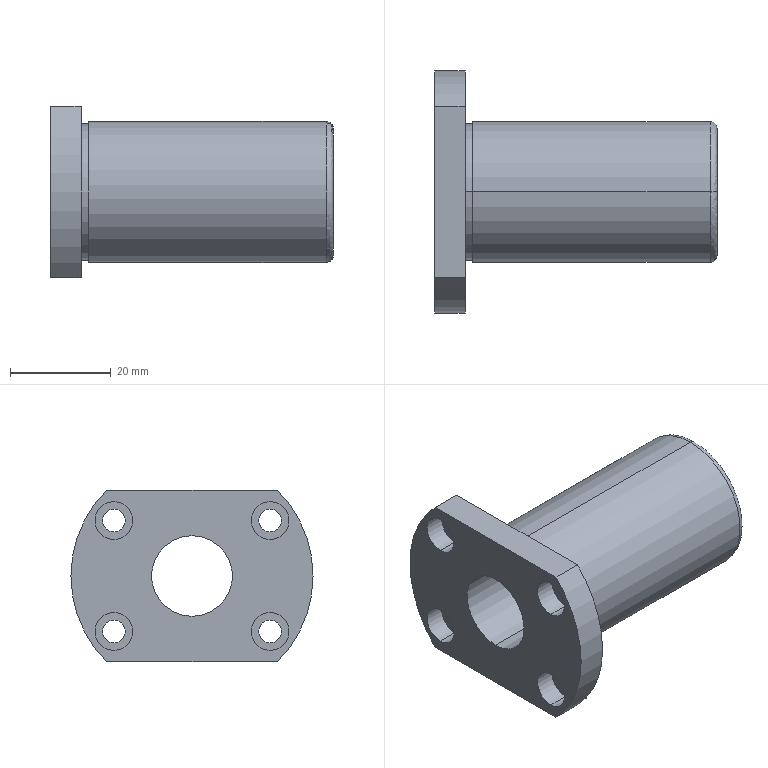Part | STEP file | LHFCD16 flanged linear bearing_LHFCD16 | 1 solid | 36 faces | box 56 x 48 x 34 mm | volume 27480 mm3 | cylinder 24 | plane 10 | spline 2 | commonest cylinder face diameters 4.5 x8 7.5 x8 16 x2 27 x2 28 x2 48 x2